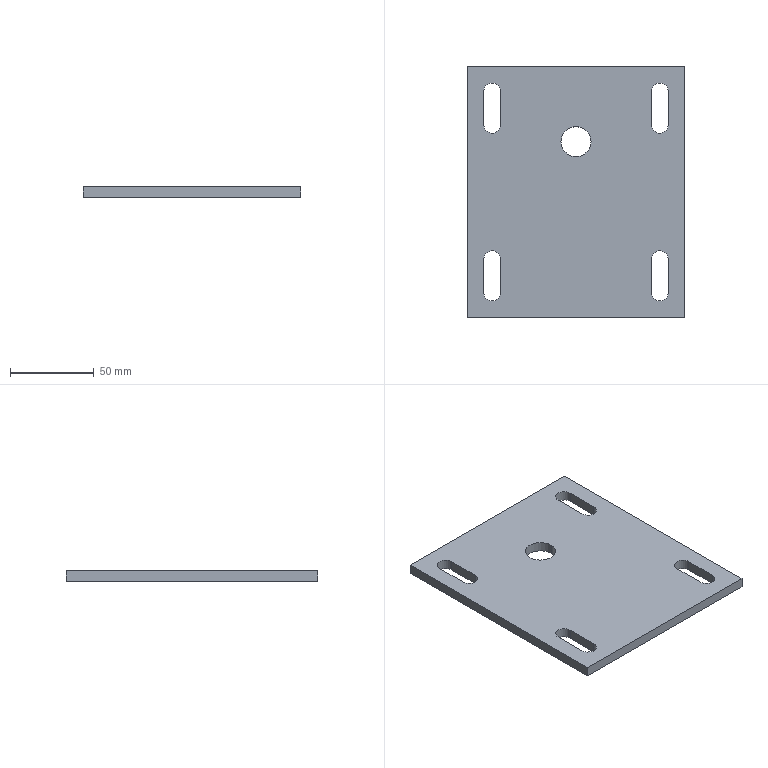Part | STEP file | 01-Seat plate 1 | 1 solid | 24 faces | box 130 x 150 x 6 mm | volume 108788 mm3 | plane 14 | cylinder 10 | commonest cylinder face diameters 10 x8 18 x2